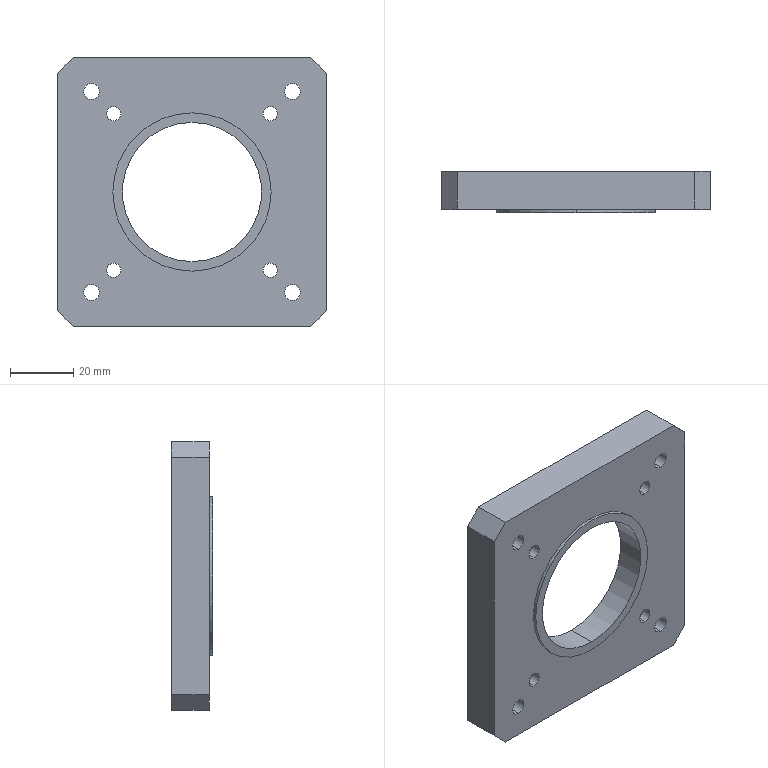Part | SolidWorks | features ICE 3, HoleWzd 2, Chamfer 1, Extrusion 1 | 1 solid | 49 faces | box 85 x 13 x 85 mm | volume 56434 mm3 | cylinder 33 | plane 16 | commonest cylinder face diameters 4.5 x8 5 x8 8 x8 70 x5 44 x2 50 x2